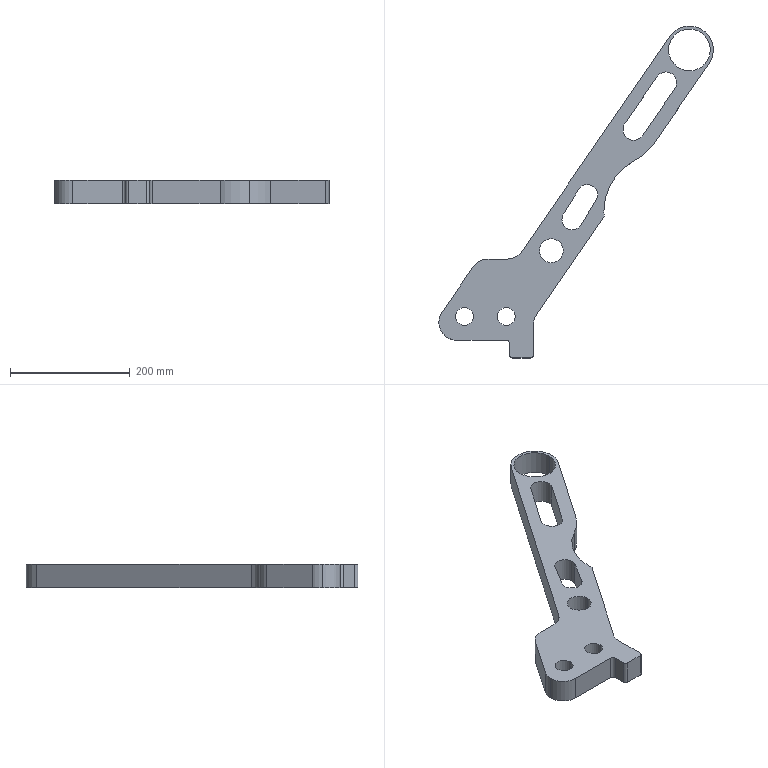Part | SolidWorks | features Extrusion 1 | 1 solid | 41 faces | box 459.333 x 555.5 x 40 mm | volume 1753830 mm3 | cylinder 26 | plane 15 | commonest cylinder face diameters 60 x5 30 x4 10 x3 35.817 x3 34.433 x2 40 x2
STEP:
#1=CARTESIAN_POINT('',(136223.495,-173373.447,40.));
#2=VERTEX_POINT('',#1);
#3=CARTESIAN_POINT('',(136220.343,-173383.593,40.));
#4=VERTEX_POINT('',#3);
#5=CARTESIAN_POINT('',(136238.252,-173383.593,40.));
#6=DIRECTION('',(0.,0.,1.));
#7=DIRECTION('',(1.,0.,0.));
#8=AXIS2_PLACEMENT_3D('',#5,#6,#7);
#9=CIRCLE('',#8,17.909);
#10=EDGE_CURVE('',#2,#4,#9,.T.);
#11=ORIENTED_EDGE('',*,*,#10,.T.);
#12=CARTESIAN_POINT('',(136220.343,-173383.593,0.));
#13=VERTEX_POINT('',#12);
#14=CARTESIAN_POINT('',(136220.343,-173383.593,40.));
#15=DIRECTION('',(0.,0.,-1.));
#16=VECTOR('',#15,1000.);
#17=LINE('',#14,#16);
#18=EDGE_CURVE('',#4,#13,#17,.T.);
#19=ORIENTED_EDGE('',*,*,#18,.T.);
#20=CARTESIAN_POINT('',(136223.495,-173373.447,0.));
#21=VERTEX_POINT('',#20);
#22=CARTESIAN_POINT('',(136238.252,-173383.593,0.));
#23=DIRECTION('',(0.,0.,1.));
#24=DIRECTION('',(1.,0.,0.));
#25=AXIS2_PLACEMENT_3D('',#22,#23,#24);
#26=CIRCLE('',#25,17.909);
#27=EDGE_CURVE('',#21,#13,#26,.T.);
#28=ORIENTED_EDGE('',*,*,#27,.F.);
#29=CARTESIAN_POINT('',(136223.495,-173373.447,40.));
#30=DIRECTION('',(0.,0.,-1.));
#31=VECTOR('',#30,1000.);
#32=LINE('',#29,#31);
#33=EDGE_CURVE('',#2,#21,#32,.T.);
#34=ORIENTED_EDGE('',*,*,#33,.F.);
#35=EDGE_LOOP('',(#11,#19,#28,#34));
#36=FACE_OUTER_BOUND('',#35,.T.);
#37=CARTESIAN_POINT('',(136238.252,-173383.593,40.));
#38=DIRECTION('',(0.,0.,-1.));
#39=DIRECTION('',(-1.,0.,0.));
#40=AXIS2_PLACEMENT_3D('',#37,#38,#39);
#41=CYLINDRICAL_SURFACE('',#40,17.909);
#42=ADVANCED_FACE('',(#36),#41,.F.);
#43=CARTESIAN_POINT('',(136121.227,-173524.21,40.));
#44=VERTEX_POINT('',#43);
#45=CARTESIAN_POINT('',(136118.026,-173534.208,40.));
#46=VERTEX_POINT('',#45);
#47=CARTESIAN_POINT('',(136135.243,-173534.208,40.));
#48=DIRECTION('',(0.,0.,1.));
#49=DIRECTION('',(1.,0.,0.));
#50=AXIS2_PLACEMENT_3D('',#47,#48,#49);
#51=CIRCLE('',#50,17.217);
#52=EDGE_CURVE('',#44,#46,#51,.T.);
#53=ORIENTED_EDGE('',*,*,#52,.T.);
#54=CARTESIAN_POINT('',(136118.026,-173534.208,0.));
#55=VERTEX_POINT('',#54);
#56=CARTESIAN_POINT('',(136118.026,-173534.208,40.));
#57=DIRECTION('',(0.,0.,-1.));
#58=VECTOR('',#57,1000.);
#59=LINE('',#56,#58);
#60=EDGE_CURVE('',#46,#55,#59,.T.);
#61=ORIENTED_EDGE('',*,*,#60,.T.);
#62=CARTESIAN_POINT('',(136121.227,-173524.21,0.));
#63=VERTEX_POINT('',#62);
#64=CARTESIAN_POINT('',(136135.243,-173534.208,0.));
#65=DIRECTION('',(0.,0.,1.));
#66=DIRECTION('',(1.,0.,0.));
#67=AXIS2_PLACEMENT_3D('',#64,#65,#66);
#68=CIRCLE('',#67,17.217);
#69=EDGE_CURVE('',#63,#55,#68,.T.);
#70=ORIENTED_EDGE('',*,*,#69,.F.);
#71=CARTESIAN_POINT('',(136121.227,-173524.21,40.));
#72=DIRECTION('',(0.,0.,-1.));
#73=VECTOR('',#72,1000.);
#74=LINE('',#71,#73);
#75=EDGE_CURVE('',#44,#63,#74,.T.);
#76=ORIENTED_EDGE('',*,*,#75,.F.);
#77=EDGE_LOOP('',(#53,#61,#70,#76));
#78=FACE_OUTER_BOUND('',#77,.T.);
#79=CARTESIAN_POINT('',(136135.243,-173534.208,40.));
#80=DIRECTION('',(0.,0.,-1.));
#81=DIRECTION('',(-1.,0.,0.));
#82=AXIS2_PLACEMENT_3D('',#79,#80,#81);
#83=CYLINDRICAL_SURFACE('',#82,17.217);
#84=ADVANCED_FACE('',(#78),#83,.F.);
#85=CARTESIAN_POINT('',(136296.441,-173250.292,40.));
#86=VERTEX_POINT('',#85);
#87=CARTESIAN_POINT('',(136366.441,-173250.292,40.));
#88=VERTEX_POINT('',#87);
#89=CARTESIAN_POINT('',(136331.441,-173250.292,40.));
#90=DIRECTION('',(0.,0.,1.));
#91=DIRECTION('',(1.,0.,0.));
#92=AXIS2_PLACEMENT_3D('',#89,#90,#91);
#93=CIRCLE('',#92,35.);
#94=EDGE_CURVE('',#86,#88,#93,.T.);
#95=ORIENTED_EDGE('',*,*,#94,.T.);
#96=CARTESIAN_POINT('',(136366.441,-173250.292,0.));
#97=VERTEX_POINT('',#96);
#98=CARTESIAN_POINT('',(136366.441,-173250.292,40.));
#99=DIRECTION('',(0.,0.,-1.));
#100=VECTOR('',#99,1000.);
#101=LINE('',#98,#100);
#102=EDGE_CURVE('',#88,#97,#101,.T.);
#103=ORIENTED_EDGE('',*,*,#102,.T.);
#104=CARTESIAN_POINT('',(136296.441,-173250.292,0.));
#105=VERTEX_POINT('',#104);
#106=CARTESIAN_POINT('',(136331.441,-173250.292,0.));
#107=DIRECTION('',(0.,0.,1.));
#108=DIRECTION('',(1.,0.,0.));
#109=AXIS2_PLACEMENT_3D('',#106,#107,#108);
#110=CIRCLE('',#109,35.);
#111=EDGE_CURVE('',#105,#97,#110,.T.);
#112=ORIENTED_EDGE('',*,*,#111,.F.);
#113=CARTESIAN_POINT('',(136296.441,-173250.292,40.));
#114=DIRECTION('',(0.,0.,-1.));
#115=VECTOR('',#114,1000.);
#116=LINE('',#113,#115);
#117=EDGE_CURVE('',#86,#105,#116,.T.);
#118=ORIENTED_EDGE('',*,*,#117,.F.);
#119=EDGE_LOOP('',(#95,#103,#112,#118));
#120=FACE_OUTER_BOUND('',#119,.T.);
#121=CARTESIAN_POINT('',(136331.441,-173250.292,40.));
#122=DIRECTION('',(0.,0.,-1.));
#123=DIRECTION('',(-1.,0.,0.));
#124=AXIS2_PLACEMENT_3D('',#121,#122,#123);
#125=CYLINDRICAL_SURFACE('',#124,35.);
#126=ADVANCED_FACE('',(#120),#125,.F.);
#127=CARTESIAN_POINT('',(136080.441,-173586.292,40.));
#128=VERTEX_POINT('',#127);
#129=CARTESIAN_POINT('',(136120.441,-173586.292,40.));
#130=VERTEX_POINT('',#129);
#131=CARTESIAN_POINT('',(136100.441,-173586.292,40.));
#132=DIRECTION('',(0.,0.,1.));
#133=DIRECTION('',(1.,0.,0.));
#134=AXIS2_PLACEMENT_3D('',#131,#132,#133);
#135=CIRCLE('',#134,20.);
#136=EDGE_CURVE('',#128,#130,#135,.T.);
#137=ORIENTED_EDGE('',*,*,#136,.T.);
#138=CARTESIAN_POINT('',(136120.441,-173586.292,0.));
#139=VERTEX_POINT('',#138);
#140=CARTESIAN_POINT('',(136120.441,-173586.292,40.));
#141=DIRECTION('',(0.,0.,-1.));
#142=VECTOR('',#141,1000.);
#143=LINE('',#140,#142);
#144=EDGE_CURVE('',#130,#139,#143,.T.);
#145=ORIENTED_EDGE('',*,*,#144,.T.);
#146=CARTESIAN_POINT('',(136080.441,-173586.292,0.));
#147=VERTEX_POINT('',#146);
#148=CARTESIAN_POINT('',(136100.441,-173586.292,0.));
#149=DIRECTION('',(0.,0.,1.));
#150=DIRECTION('',(1.,0.,0.));
#151=AXIS2_PLACEMENT_3D('',#148,#149,#150);
#152=CIRCLE('',#151,20.);
#153=EDGE_CURVE('',#147,#139,#152,.T.);
#154=ORIENTED_EDGE('',*,*,#153,.F.);
#155=CARTESIAN_POINT('',(136080.441,-173586.292,40.));
#156=DIRECTION('',(0.,0.,-1.));
#157=VECTOR('',#156,1000.);
#158=LINE('',#155,#157);
#159=EDGE_CURVE('',#128,#147,#158,.T.);
#160=ORIENTED_EDGE('',*,*,#159,.F.);
#161=EDGE_LOOP('',(#137,#145,#154,#160));
#162=FACE_OUTER_BOUND('',#161,.T.);
#163=CARTESIAN_POINT('',(136100.441,-173586.292,40.));
#164=DIRECTION('',(0.,0.,-1.));
#165=DIRECTION('',(-1.,0.,0.));
#166=AXIS2_PLACEMENT_3D('',#163,#164,#165);
#167=CYLINDRICAL_SURFACE('',#166,20.);
#168=ADVANCED_FACE('',(#162),#167,.F.);
#169=CARTESIAN_POINT('',(135939.816,-173696.292,40.));
#170=VERTEX_POINT('',#169);
#171=CARTESIAN_POINT('',(135969.816,-173696.292,40.));
#172=VERTEX_POINT('',#171);
#173=CARTESIAN_POINT('',(135954.816,-173696.292,40.));
#174=DIRECTION('',(0.,0.,1.));
#175=DIRECTION('',(1.,0.,0.));
#176=AXIS2_PLACEMENT_3D('',#173,#174,#175);
#177=CIRCLE('',#176,15.);
#178=EDGE_CURVE('',#170,#172,#177,.T.);
#179=ORIENTED_EDGE('',*,*,#178,.T.);
#180=CARTESIAN_POINT('',(135969.816,-173696.292,0.));
#181=VERTEX_POINT('',#180);
#182=CARTESIAN_POINT('',(135969.816,-173696.292,40.));
#183=DIRECTION('',(0.,0.,-1.));
#184=VECTOR('',#183,1000.);
#185=LINE('',#182,#184);
#186=EDGE_CURVE('',#172,#181,#185,.T.);
#187=ORIENTED_EDGE('',*,*,#186,.T.);
#188=CARTESIAN_POINT('',(135939.816,-173696.292,0.));
#189=VERTEX_POINT('',#188);
#190=CARTESIAN_POINT('',(135954.816,-173696.292,0.));
#191=DIRECTION('',(0.,0.,1.));
#192=DIRECTION('',(1.,0.,0.));
#193=AXIS2_PLACEMENT_3D('',#190,#191,#192);
#194=CIRCLE('',#193,15.);
#195=EDGE_CURVE('',#189,#181,#194,.T.);
#196=ORIENTED_EDGE('',*,*,#195,.F.);
#197=CARTESIAN_POINT('',(135939.816,-173696.292,40.));
#198=DIRECTION('',(0.,0.,-1.));
#199=VECTOR('',#198,1000.);
#200=LINE('',#197,#199);
#201=EDGE_CURVE('',#170,#189,#200,.T.);
#202=ORIENTED_EDGE('',*,*,#201,.F.);
#203=EDGE_LOOP('',(#179,#187,#196,#202));
#204=FACE_OUTER_BOUND('',#203,.T.);
#205=CARTESIAN_POINT('',(135954.816,-173696.292,40.));
#206=DIRECTION('',(0.,0.,-1.));
#207=DIRECTION('',(-1.,0.,0.));
#208=AXIS2_PLACEMENT_3D('',#205,#206,#207);
#209=CYLINDRICAL_SURFACE('',#208,15.);
#210=ADVANCED_FACE('',(#204),#209,.F.);
#211=CARTESIAN_POINT('',(136009.816,-173696.292,40.));
#212=VERTEX_POINT('',#211);
#213=CARTESIAN_POINT('',(136039.816,-173696.292,40.));
#214=VERTEX_POINT('',#213);
#215=CARTESIAN_POINT('',(136024.816,-173696.292,40.));
#216=DIRECTION('',(0.,0.,1.));
#217=DIRECTION('',(1.,0.,0.));
#218=AXIS2_PLACEMENT_3D('',#215,#216,#217);
#219=CIRCLE('',#218,15.);
#220=EDGE_CURVE('',#212,#214,#219,.T.);
#221=ORIENTED_EDGE('',*,*,#220,.T.);
#222=CARTESIAN_POINT('',(136039.816,-173696.292,0.));
#223=VERTEX_POINT('',#222);
#224=CARTESIAN_POINT('',(136039.816,-173696.292,40.));
#225=DIRECTION('',(0.,0.,-1.));
#226=VECTOR('',#225,1000.);
#227=LINE('',#224,#226);
#228=EDGE_CURVE('',#214,#223,#227,.T.);
#229=ORIENTED_EDGE('',*,*,#228,.T.);
#230=CARTESIAN_POINT('',(136009.816,-173696.292,0.));
#231=VERTEX_POINT('',#230);
#232=CARTESIAN_POINT('',(136024.816,-173696.292,0.));
#233=DIRECTION('',(0.,0.,1.));
#234=DIRECTION('',(1.,0.,0.));
#235=AXIS2_PLACEMENT_3D('',#232,#233,#234);
#236=CIRCLE('',#235,15.);
#237=EDGE_CURVE('',#231,#223,#236,.T.);
#238=ORIENTED_EDGE('',*,*,#237,.F.);
#239=CARTESIAN_POINT('',(136009.816,-173696.292,40.));
#240=DIRECTION('',(0.,0.,-1.));
#241=VECTOR('',#240,1000.);
#242=LINE('',#239,#241);
#243=EDGE_CURVE('',#212,#231,#242,.T.);
#244=ORIENTED_EDGE('',*,*,#243,.F.);
#245=EDGE_LOOP('',(#221,#229,#238,#244));
#246=FACE_OUTER_BOUND('',#245,.T.);
#247=CARTESIAN_POINT('',(136024.816,-173696.292,40.));
#248=DIRECTION('',(0.,0.,-1.));
#249=DIRECTION('',(-1.,0.,0.));
#250=AXIS2_PLACEMENT_3D('',#247,#248,#249);
#251=CYLINDRICAL_SURFACE('',#250,15.);
#252=ADVANCED_FACE('',(#246),#251,.F.);
#253=CARTESIAN_POINT('',(136188.379,-173519.712,40.));
#254=VERTEX_POINT('',#253);
#255=CARTESIAN_POINT('',(136238.252,-173436.604,40.));
#256=VERTEX_POINT('',#255);
#257=CARTESIAN_POINT('',(136282.56,-173519.712,40.));
#258=DIRECTION('',(0.,0.,-1.));
#259=DIRECTION('',(-1.,0.,0.));
#260=AXIS2_PLACEMENT_3D('',#257,#258,#259);
#261=CIRCLE('',#260,94.181);
#262=EDGE_CURVE('',#254,#256,#261,.T.);
#263=ORIENTED_EDGE('',*,*,#262,.F.);
#264=CARTESIAN_POINT('',(136188.379,-173519.712,0.));
#265=VERTEX_POINT('',#264);
#266=CARTESIAN_POINT('',(136188.379,-173519.712,40.));
#267=DIRECTION('',(0.,0.,-1.));
#268=VECTOR('',#267,1000.);
#269=LINE('',#266,#268);
#270=EDGE_CURVE('',#254,#265,#269,.T.);
#271=ORIENTED_EDGE('',*,*,#270,.T.);
#272=CARTESIAN_POINT('',(136238.252,-173436.604,0.));
#273=VERTEX_POINT('',#272);
#274=CARTESIAN_POINT('',(136282.56,-173519.712,0.));
#275=DIRECTION('',(0.,0.,-1.));
#276=DIRECTION('',(-1.,0.,0.));
#277=AXIS2_PLACEMENT_3D('',#274,#275,#276);
#278=CIRCLE('',#277,94.181);
#279=EDGE_CURVE('',#265,#273,#278,.T.);
#280=ORIENTED_EDGE('',*,*,#279,.T.);
#281=CARTESIAN_POINT('',(136238.252,-173436.604,40.));
#282=DIRECTION('',(0.,0.,-1.));
#283=VECTOR('',#282,1000.);
#284=LINE('',#281,#283);
#285=EDGE_CURVE('',#256,#273,#284,.T.);
#286=ORIENTED_EDGE('',*,*,#285,.F.);
#287=EDGE_LOOP('',(#263,#271,#280,#286));
#288=FACE_OUTER_BOUND('',#287,.T.);
#289=CARTESIAN_POINT('',(136282.56,-173519.712,40.));
#290=DIRECTION('',(0.,0.,-1.));
#291=DIRECTION('',(-1.,0.,0.));
#292=AXIS2_PLACEMENT_3D('',#289,#290,#291);
#293=CYLINDRICAL_SURFACE('',#292,94.181);
#294=ADVANCED_FACE('',(#288),#293,.F.);
#295=CARTESIAN_POINT('',(135912.108,-173706.292,40.));
#296=VERTEX_POINT('',#295);
#297=CARTESIAN_POINT('',(135942.108,-173736.292,40.));
#298=VERTEX_POINT('',#297);
#299=CARTESIAN_POINT('',(135942.108,-173706.292,40.));
#300=DIRECTION('',(0.,0.,1.));
#301=DIRECTION('',(1.,0.,0.));
#302=AXIS2_PLACEMENT_3D('',#299,#300,#301);
#303=CIRCLE('',#302,30.);
#304=EDGE_CURVE('',#296,#298,#303,.T.);
#305=ORIENTED_EDGE('',*,*,#304,.F.);
#306=CARTESIAN_POINT('',(135912.108,-173706.292,0.));
#307=VERTEX_POINT('',#306);
#308=CARTESIAN_POINT('',(135912.108,-173706.292,40.));
#309=DIRECTION('',(0.,0.,-1.));
#310=VECTOR('',#309,1000.);
#311=LINE('',#308,#310);
#312=EDGE_CURVE('',#296,#307,#311,.T.);
#313=ORIENTED_EDGE('',*,*,#312,.T.);
#314=CARTESIAN_POINT('',(135942.108,-173736.292,0.));
#315=VERTEX_POINT('',#314);
#316=CARTESIAN_POINT('',(135942.108,-173706.292,0.));
#317=DIRECTION('',(0.,0.,1.));
#318=DIRECTION('',(1.,0.,0.));
#319=AXIS2_PLACEMENT_3D('',#316,#317,#318);
#320=CIRCLE('',#319,30.);
#321=EDGE_CURVE('',#307,#315,#320,.T.);
#322=ORIENTED_EDGE('',*,*,#321,.T.);
#323=CARTESIAN_POINT('',(135942.108,-173736.292,40.));
#324=DIRECTION('',(0.,0.,-1.));
#325=VECTOR('',#324,1000.);
#326=LINE('',#323,#325);
#327=EDGE_CURVE('',#298,#315,#326,.T.);
#328=ORIENTED_EDGE('',*,*,#327,.F.);
#329=EDGE_LOOP('',(#305,#313,#322,#328));
#330=FACE_OUTER_BOUND('',#329,.T.);
#331=CARTESIAN_POINT('',(135942.108,-173706.292,40.));
#332=DIRECTION('',(0.,0.,-1.));
#333=DIRECTION('',(-1.,0.,0.));
#334=AXIS2_PLACEMENT_3D('',#331,#332,#333);
#335=CYLINDRICAL_SURFACE('',#334,30.);
#336=ADVANCED_FACE('',(#330),#335,.T.);
#337=ORIENTED_EDGE('',*,*,#136,.F.);
#338=CARTESIAN_POINT('',(136100.441,-173586.292,40.));
#339=DIRECTION('',(0.,0.,1.));
#340=DIRECTION('',(1.,0.,0.));
#341=AXIS2_PLACEMENT_3D('',#338,#339,#340);
#342=CIRCLE('',#341,20.);
#343=EDGE_CURVE('',#130,#128,#342,.T.);
#344=ORIENTED_EDGE('',*,*,#343,.F.);
#345=EDGE_LOOP('',(#337,#344));
#346=FACE_BOUND('',#345,.T.);
#347=ORIENTED_EDGE('',*,*,#220,.F.);
#348=CARTESIAN_POINT('',(136024.816,-173696.292,40.));
#349=DIRECTION('',(0.,0.,1.));
#350=DIRECTION('',(1.,0.,0.));
#351=AXIS2_PLACEMENT_3D('',#348,#349,#350);
#352=CIRCLE('',#351,15.);
#353=EDGE_CURVE('',#214,#212,#352,.T.);
#354=ORIENTED_EDGE('',*,*,#353,.F.);
#355=EDGE_LOOP('',(#347,#354));
#356=FACE_BOUND('',#355,.T.);
#357=CARTESIAN_POINT('',(136364.403,-173272.954,40.));
#358=VERTEX_POINT('',#357);
#359=CARTESIAN_POINT('',(136298.479,-173227.631,40.));
#360=VERTEX_POINT('',#359);
#361=CARTESIAN_POINT('',(136331.441,-173250.292,40.));
#362=DIRECTION('',(0.,0.,1.));
#363=DIRECTION('',(1.,0.,0.));
#364=AXIS2_PLACEMENT_3D('',#361,#362,#363);
#365=CIRCLE('',#364,40.);
#366=EDGE_CURVE('',#358,#360,#365,.T.);
#367=ORIENTED_EDGE('',*,*,#366,.T.);
#368=CARTESIAN_POINT('',(136051.215,-173587.288,40.));
#369=VERTEX_POINT('',#368);
#370=CARTESIAN_POINT('',(136298.479,-173227.631,40.));
#371=DIRECTION('',(-0.5665,-0.824,0.));
#372=VECTOR('',#371,1000.);
#373=LINE('',#370,#372);
#374=EDGE_CURVE('',#360,#369,#373,.T.);
#375=ORIENTED_EDGE('',*,*,#374,.T.);
#376=CARTESIAN_POINT('',(136026.494,-173600.292,40.));
#377=VERTEX_POINT('',#376);
#378=CARTESIAN_POINT('',(136026.494,-173570.292,40.));
#379=DIRECTION('',(0.,0.,-1.));
#380=DIRECTION('',(1.,0.,0.));
#381=AXIS2_PLACEMENT_3D('',#378,#379,#380);
#382=CIRCLE('',#381,30.);
#383=EDGE_CURVE('',#369,#377,#382,.T.);
#384=ORIENTED_EDGE('',*,*,#383,.T.);
#385=CARTESIAN_POINT('',(135994.358,-173600.292,40.));
#386=VERTEX_POINT('',#385);
#387=CARTESIAN_POINT('',(135994.358,-173600.292,40.));
#388=DIRECTION('',(-1.,0.,0.));
#389=VECTOR('',#388,1000.);
#390=LINE('',#387,#389);
#391=EDGE_CURVE('',#377,#386,#390,.T.);
#392=ORIENTED_EDGE('',*,*,#391,.T.);
#393=CARTESIAN_POINT('',(135969.637,-173613.297,40.));
#394=VERTEX_POINT('',#393);
#395=CARTESIAN_POINT('',(135994.358,-173630.292,40.));
#396=DIRECTION('',(0.,0.,1.));
#397=DIRECTION('',(1.,0.,0.));
#398=AXIS2_PLACEMENT_3D('',#395,#396,#397);
#399=CIRCLE('',#398,30.);
#400=EDGE_CURVE('',#386,#394,#399,.T.);
#401=ORIENTED_EDGE('',*,*,#400,.T.);
#402=CARTESIAN_POINT('',(135917.387,-173689.297,40.));
#403=VERTEX_POINT('',#402);
#404=CARTESIAN_POINT('',(135969.637,-173613.297,40.));
#405=DIRECTION('',(-0.5665,-0.824,0.));
#406=VECTOR('',#405,1000.);
#407=LINE('',#404,#406);
#408=EDGE_CURVE('',#394,#403,#407,.T.);
#409=ORIENTED_EDGE('',*,*,#408,.T.);
#410=CARTESIAN_POINT('',(135942.108,-173706.292,40.));
#411=DIRECTION('',(0.,0.,1.));
#412=DIRECTION('',(1.,0.,0.));
#413=AXIS2_PLACEMENT_3D('',#410,#411,#412);
#414=CIRCLE('',#413,30.);
#415=EDGE_CURVE('',#403,#296,#414,.T.);
#416=ORIENTED_EDGE('',*,*,#415,.T.);
#417=ORIENTED_EDGE('',*,*,#304,.T.);
#418=CARTESIAN_POINT('',(136025.441,-173736.292,40.));
#419=VERTEX_POINT('',#418);
#420=CARTESIAN_POINT('',(135942.108,-173736.292,40.));
#421=DIRECTION('',(1.,0.,0.));
#422=VECTOR('',#421,1000.);
#423=LINE('',#420,#422);
#424=EDGE_CURVE('',#298,#419,#423,.T.);
#425=ORIENTED_EDGE('',*,*,#424,.T.);
#426=CARTESIAN_POINT('',(136030.441,-173741.292,40.));
#427=VERTEX_POINT('',#426);
#428=CARTESIAN_POINT('',(136025.441,-173741.292,40.));
#429=DIRECTION('',(0.,0.,-1.));
#430=DIRECTION('',(1.,0.,0.));
#431=AXIS2_PLACEMENT_3D('',#428,#429,#430);
#432=CIRCLE('',#431,5.);
#433=EDGE_CURVE('',#419,#427,#432,.T.);
#434=ORIENTED_EDGE('',*,*,#433,.T.);
#435=CARTESIAN_POINT('',(136030.441,-173760.792,40.));
#436=VERTEX_POINT('',#435);
#437=CARTESIAN_POINT('',(136030.441,-173760.792,40.));
#438=DIRECTION('',(0.,-1.,0.));
#439=VECTOR('',#438,1000.);
#440=LINE('',#437,#439);
#441=EDGE_CURVE('',#427,#436,#440,.T.);
#442=ORIENTED_EDGE('',*,*,#441,.T.);
#443=CARTESIAN_POINT('',(136035.441,-173765.792,40.));
#444=VERTEX_POINT('',#443);
#445=CARTESIAN_POINT('',(136035.441,-173760.792,40.));
#446=DIRECTION('',(0.,0.,1.));
#447=DIRECTION('',(1.,0.,0.));
#448=AXIS2_PLACEMENT_3D('',#445,#446,#447);
#449=CIRCLE('',#448,5.);
#450=EDGE_CURVE('',#436,#444,#449,.T.);
#451=ORIENTED_EDGE('',*,*,#450,.T.);
#452=CARTESIAN_POINT('',(136065.441,-173765.792,40.));
#453=VERTEX_POINT('',#452);
#454=CARTESIAN_POINT('',(136035.441,-173765.792,40.));
#455=DIRECTION('',(1.,0.,0.));
#456=VECTOR('',#455,1000.);
#457=LINE('',#454,#456);
#458=EDGE_CURVE('',#444,#453,#457,.T.);
#459=ORIENTED_EDGE('',*,*,#458,.T.);
#460=CARTESIAN_POINT('',(136070.441,-173760.792,40.));
#461=VERTEX_POINT('',#460);
#462=CARTESIAN_POINT('',(136065.441,-173760.792,40.));
#463=DIRECTION('',(0.,0.,1.));
#464=DIRECTION('',(1.,0.,0.));
#465=AXIS2_PLACEMENT_3D('',#462,#463,#464);
#466=CIRCLE('',#465,5.);
#467=EDGE_CURVE('',#453,#461,#466,.T.);
#468=ORIENTED_EDGE('',*,*,#467,.T.);
#469=CARTESIAN_POINT('',(136070.441,-173709.852,40.));
#470=VERTEX_POINT('',#469);
#471=CARTESIAN_POINT('',(136070.441,-173760.792,40.));
#472=DIRECTION('',(0.,1.,0.));
#473=VECTOR('',#472,1000.);
#474=LINE('',#471,#473);
#475=EDGE_CURVE('',#461,#470,#474,.T.);
#476=ORIENTED_EDGE('',*,*,#475,.T.);
#477=CARTESIAN_POINT('',(136075.72,-173692.856,40.));
#478=VERTEX_POINT('',#477);
#479=CARTESIAN_POINT('',(136100.441,-173709.852,40.));
#480=DIRECTION('',(0.,0.,-1.));
#481=DIRECTION('',(1.,0.,0.));
#482=AXIS2_PLACEMENT_3D('',#479,#480,#481);
#483=CIRCLE('',#482,30.);
#484=EDGE_CURVE('',#470,#478,#483,.T.);
#485=ORIENTED_EDGE('',*,*,#484,.T.);
#486=CARTESIAN_POINT('',(136188.781,-173528.403,40.));
#487=VERTEX_POINT('',#486);
#488=CARTESIAN_POINT('',(136188.781,-173528.403,40.));
#489=DIRECTION('',(0.5665,0.824,0.));
#490=VECTOR('',#489,1000.);
#491=LINE('',#488,#490);
#492=EDGE_CURVE('',#478,#487,#491,.T.);
#493=ORIENTED_EDGE('',*,*,#492,.T.);
#494=CARTESIAN_POINT('',(136282.56,-173519.712,40.));
#495=DIRECTION('',(0.,0.,-1.));
#496=DIRECTION('',(-1.,0.,0.));
#497=AXIS2_PLACEMENT_3D('',#494,#495,#496);
#498=CIRCLE('',#497,94.181);
#499=EDGE_CURVE('',#487,#254,#498,.T.);
#500=ORIENTED_EDGE('',*,*,#499,.T.);
#501=ORIENTED_EDGE('',*,*,#262,.T.);
#502=CARTESIAN_POINT('',(136273.61,-173405.015,40.));
#503=VERTEX_POINT('',#502);
#504=CARTESIAN_POINT('',(136191.206,-173348.362,40.));
#505=DIRECTION('',(0.,0.,1.));
#506=DIRECTION('',(1.,0.,0.));
#507=AXIS2_PLACEMENT_3D('',#504,#505,#506);
#508=CIRCLE('',#507,100.);
#509=EDGE_CURVE('',#256,#503,#508,.T.);
#510=ORIENTED_EDGE('',*,*,#509,.T.);
#511=CARTESIAN_POINT('',(136364.403,-173272.954,40.));
#512=DIRECTION('',(0.5665,0.824,0.));
#513=VECTOR('',#512,1000.);
#514=LINE('',#511,#513);
#515=EDGE_CURVE('',#503,#358,#514,.T.);
#516=ORIENTED_EDGE('',*,*,#515,.T.);
#517=EDGE_LOOP('',(#367,#375,#384,#392,#401,#409,#416,#417,#425,#434,#442,#451,#459,#468,#476,#485,#493,#500,#501,#510,#516));
#518=FACE_OUTER_BOUND('',#517,.T.);
#519=ORIENTED_EDGE('',*,*,#178,.F.);
#520=CARTESIAN_POINT('',(135954.816,-173696.292,40.));
#521=DIRECTION('',(0.,0.,1.));
#522=DIRECTION('',(1.,0.,0.));
#523=AXIS2_PLACEMENT_3D('',#520,#521,#522);
#524=CIRCLE('',#523,15.);
#525=EDGE_CURVE('',#172,#170,#524,.T.);
#526=ORIENTED_EDGE('',*,*,#525,.F.);
#527=EDGE_LOOP('',(#519,#526));
#528=FACE_BOUND('',#527,.T.);
#529=ORIENTED_EDGE('',*,*,#94,.F.);
#530=CARTESIAN_POINT('',(136331.441,-173250.292,40.));
#531=DIRECTION('',(0.,0.,1.));
#532=DIRECTION('',(1.,0.,0.));
#533=AXIS2_PLACEMENT_3D('',#530,#531,#532);
#534=CIRCLE('',#533,35.);
#535=EDGE_CURVE('',#88,#86,#534,.T.);
#536=ORIENTED_EDGE('',*,*,#535,.F.);
#537=EDGE_LOOP('',(#529,#536));
#538=FACE_BOUND('',#537,.T.);
#539=CARTESIAN_POINT('',(136150.474,-173542.235,40.));
#540=VERTEX_POINT('',#539);
#541=CARTESIAN_POINT('',(136175.848,-173500.774,40.));
#542=VERTEX_POINT('',#541);
#543=CARTESIAN_POINT('',(136150.474,-173542.235,40.));
#544=DIRECTION('',(0.522,0.8529,0.));
#545=VECTOR('',#544,1000.);
#546=LINE('',#543,#545);
#547=EDGE_CURVE('',#540,#542,#546,.T.);
#548=ORIENTED_EDGE('',*,*,#547,.F.);
#549=CARTESIAN_POINT('',(136135.243,-173534.208,40.));
#550=DIRECTION('',(0.,0.,1.));
#551=DIRECTION('',(1.,0.,0.));
#552=AXIS2_PLACEMENT_3D('',#549,#550,#551);
#553=CIRCLE('',#552,17.217);
#554=EDGE_CURVE('',#46,#540,#553,.T.);
#555=ORIENTED_EDGE('',*,*,#554,.F.);
#556=ORIENTED_EDGE('',*,*,#52,.F.);
#557=CARTESIAN_POINT('',(136146.694,-173482.736,40.));
#558=VERTEX_POINT('',#557);
#559=CARTESIAN_POINT('',(136121.227,-173524.21,40.));
#560=DIRECTION('',(-0.5233,-0.8522,0.));
#561=VECTOR('',#560,1000.);
#562=LINE('',#559,#561);
#563=EDGE_CURVE('',#558,#44,#562,.T.);
#564=ORIENTED_EDGE('',*,*,#563,.F.);
#565=CARTESIAN_POINT('',(136160.639,-173492.777,40.));
#566=DIRECTION('',(0.,0.,1.));
#567=DIRECTION('',(1.,0.,0.));
#568=AXIS2_PLACEMENT_3D('',#565,#566,#567);
#569=CIRCLE('',#568,17.184);
#570=EDGE_CURVE('',#542,#558,#569,.T.);
#571=ORIENTED_EDGE('',*,*,#570,.F.);
#572=EDGE_LOOP('',(#548,#555,#556,#564,#571));
#573=FACE_BOUND('',#572,.T.);
#574=CARTESIAN_POINT('',(136253.009,-173393.739,40.));
#575=VERTEX_POINT('',#574);
#576=CARTESIAN_POINT('',(136306.988,-173315.224,40.));
#577=VERTEX_POINT('',#576);
#578=CARTESIAN_POINT('',(136253.009,-173393.739,40.));
#579=DIRECTION('',(0.5665,0.824,0.));
#580=VECTOR('',#579,1000.);
#581=LINE('',#578,#580);
#582=EDGE_CURVE('',#575,#577,#581,.T.);
#583=ORIENTED_EDGE('',*,*,#582,.F.);
#584=CARTESIAN_POINT('',(136238.252,-173383.593,40.));
#585=DIRECTION('',(0.,0.,1.));
#586=DIRECTION('',(1.,0.,0.));
#587=AXIS2_PLACEMENT_3D('',#584,#585,#586);
#588=CIRCLE('',#587,17.909);
#589=EDGE_CURVE('',#4,#575,#588,.T.);
#590=ORIENTED_EDGE('',*,*,#589,.F.);
#591=ORIENTED_EDGE('',*,*,#10,.F.);
#592=CARTESIAN_POINT('',(136277.474,-173294.933,40.));
#593=VERTEX_POINT('',#592);
#594=CARTESIAN_POINT('',(136223.495,-173373.447,40.));
#595=DIRECTION('',(-0.5665,-0.824,0.));
#596=VECTOR('',#595,1000.);
#597=LINE('',#594,#596);
#598=EDGE_CURVE('',#593,#2,#597,.T.);
#599=ORIENTED_EDGE('',*,*,#598,.F.);
#600=CARTESIAN_POINT('',(136292.231,-173305.078,40.));
#601=DIRECTION('',(0.,0.,1.));
#602=DIRECTION('',(1.,0.,0.));
#603=AXIS2_PLACEMENT_3D('',#600,#601,#602);
#604=CIRCLE('',#603,17.909);
#605=EDGE_CURVE('',#577,#593,#604,.T.);
#606=ORIENTED_EDGE('',*,*,#605,.F.);
#607=EDGE_LOOP('',(#583,#590,#591,#599,#606));
#608=FACE_BOUND('',#607,.T.);
#609=CARTESIAN_POINT('',(136331.441,-173250.292,40.));
#610=DIRECTION('',(0.,0.,1.));
#611=DIRECTION('',(1.,0.,0.));
#612=AXIS2_PLACEMENT_3D('',#609,#610,#611);
#613=PLANE('',#612);
#614=ADVANCED_FACE('',(#346,#356,#518,#528,#538,#573,#608),#613,.T.);
#615=ORIENTED_EDGE('',*,*,#69,.T.);
#616=CARTESIAN_POINT('',(136150.474,-173542.235,0.));
#617=VERTEX_POINT('',#616);
#618=CARTESIAN_POINT('',(136135.243,-173534.208,0.));
#619=DIRECTION('',(0.,0.,1.));
#620=DIRECTION('',(1.,0.,0.));
#621=AXIS2_PLACEMENT_3D('',#618,#619,#620);
#622=CIRCLE('',#621,17.217);
#623=EDGE_CURVE('',#55,#617,#622,.T.);
#624=ORIENTED_EDGE('',*,*,#623,.T.);
#625=CARTESIAN_POINT('',(136175.848,-173500.774,0.));
#626=VERTEX_POINT('',#625);
#627=CARTESIAN_POINT('',(136150.474,-173542.235,0.));
#628=DIRECTION('',(0.522,0.8529,0.));
#629=VECTOR('',#628,1000.);
#630=LINE('',#627,#629);
#631=EDGE_CURVE('',#617,#626,#630,.T.);
#632=ORIENTED_EDGE('',*,*,#631,.T.);
#633=CARTESIAN_POINT('',(136146.694,-173482.736,0.));
#634=VERTEX_POINT('',#633);
#635=CARTESIAN_POINT('',(136160.639,-173492.777,0.));
#636=DIRECTION('',(0.,0.,1.));
#637=DIRECTION('',(1.,0.,0.));
#638=AXIS2_PLACEMENT_3D('',#635,#636,#637);
#639=CIRCLE('',#638,17.184);
#640=EDGE_CURVE('',#626,#634,#639,.T.);
#641=ORIENTED_EDGE('',*,*,#640,.T.);
#642=CARTESIAN_POINT('',(136121.227,-173524.21,0.));
#643=DIRECTION('',(-0.5233,-0.8522,0.));
#644=VECTOR('',#643,1000.);
#645=LINE('',#642,#644);
#646=EDGE_CURVE('',#634,#63,#645,.T.);
#647=ORIENTED_EDGE('',*,*,#646,.T.);
#648=EDGE_LOOP('',(#615,#624,#632,#641,#647));
#649=FACE_BOUND('',#648,.T.);
#650=CARTESIAN_POINT('',(136364.403,-173272.954,0.));
#651=VERTEX_POINT('',#650);
#652=CARTESIAN_POINT('',(136298.479,-173227.631,0.));
#653=VERTEX_POINT('',#652);
#654=CARTESIAN_POINT('',(136331.441,-173250.292,0.));
#655=DIRECTION('',(0.,0.,1.));
#656=DIRECTION('',(1.,0.,0.));
#657=AXIS2_PLACEMENT_3D('',#654,#655,#656);
#658=CIRCLE('',#657,40.);
#659=EDGE_CURVE('',#651,#653,#658,.T.);
#660=ORIENTED_EDGE('',*,*,#659,.F.);
#661=CARTESIAN_POINT('',(136273.61,-173405.015,0.));
#662=VERTEX_POINT('',#661);
#663=CARTESIAN_POINT('',(136364.403,-173272.954,0.));
#664=DIRECTION('',(0.5665,0.824,0.));
#665=VECTOR('',#664,1000.);
#666=LINE('',#663,#665);
#667=EDGE_CURVE('',#662,#651,#666,.T.);
#668=ORIENTED_EDGE('',*,*,#667,.F.);
#669=CARTESIAN_POINT('',(136191.206,-173348.362,0.));
#670=DIRECTION('',(0.,0.,1.));
#671=DIRECTION('',(1.,0.,0.));
#672=AXIS2_PLACEMENT_3D('',#669,#670,#671);
#673=CIRCLE('',#672,100.);
#674=EDGE_CURVE('',#273,#662,#673,.T.);
#675=ORIENTED_EDGE('',*,*,#674,.F.);
#676=ORIENTED_EDGE('',*,*,#279,.F.);
#677=CARTESIAN_POINT('',(136188.781,-173528.403,0.));
#678=VERTEX_POINT('',#677);
#679=CARTESIAN_POINT('',(136282.56,-173519.712,0.));
#680=DIRECTION('',(0.,0.,-1.));
#681=DIRECTION('',(-1.,0.,0.));
#682=AXIS2_PLACEMENT_3D('',#679,#680,#681);
#683=CIRCLE('',#682,94.181);
#684=EDGE_CURVE('',#678,#265,#683,.T.);
#685=ORIENTED_EDGE('',*,*,#684,.F.);
#686=CARTESIAN_POINT('',(136075.72,-173692.856,0.));
#687=VERTEX_POINT('',#686);
#688=CARTESIAN_POINT('',(136188.781,-173528.403,0.));
#689=DIRECTION('',(0.5665,0.824,0.));
#690=VECTOR('',#689,1000.);
#691=LINE('',#688,#690);
#692=EDGE_CURVE('',#687,#678,#691,.T.);
#693=ORIENTED_EDGE('',*,*,#692,.F.);
#694=CARTESIAN_POINT('',(136070.441,-173709.852,0.));
#695=VERTEX_POINT('',#694);
#696=CARTESIAN_POINT('',(136100.441,-173709.852,0.));
#697=DIRECTION('',(0.,0.,-1.));
#698=DIRECTION('',(1.,0.,0.));
#699=AXIS2_PLACEMENT_3D('',#696,#697,#698);
#700=CIRCLE('',#699,30.);
#701=EDGE_CURVE('',#695,#687,#700,.T.);
#702=ORIENTED_EDGE('',*,*,#701,.F.);
#703=CARTESIAN_POINT('',(136070.441,-173760.792,0.));
#704=VERTEX_POINT('',#703);
#705=CARTESIAN_POINT('',(136070.441,-173760.792,0.));
#706=DIRECTION('',(0.,1.,0.));
#707=VECTOR('',#706,1000.);
#708=LINE('',#705,#707);
#709=EDGE_CURVE('',#704,#695,#708,.T.);
#710=ORIENTED_EDGE('',*,*,#709,.F.);
#711=CARTESIAN_POINT('',(136065.441,-173765.792,0.));
#712=VERTEX_POINT('',#711);
#713=CARTESIAN_POINT('',(136065.441,-173760.792,0.));
#714=DIRECTION('',(0.,0.,1.));
#715=DIRECTION('',(1.,0.,0.));
#716=AXIS2_PLACEMENT_3D('',#713,#714,#715);
#717=CIRCLE('',#716,5.);
#718=EDGE_CURVE('',#712,#704,#717,.T.);
#719=ORIENTED_EDGE('',*,*,#718,.F.);
#720=CARTESIAN_POINT('',(136035.441,-173765.792,0.));
#721=VERTEX_POINT('',#720);
#722=CARTESIAN_POINT('',(136035.441,-173765.792,0.));
#723=DIRECTION('',(1.,0.,0.));
#724=VECTOR('',#723,1000.);
#725=LINE('',#722,#724);
#726=EDGE_CURVE('',#721,#712,#725,.T.);
#727=ORIENTED_EDGE('',*,*,#726,.F.);
#728=CARTESIAN_POINT('',(136030.441,-173760.792,0.));
#729=VERTEX_POINT('',#728);
#730=CARTESIAN_POINT('',(136035.441,-173760.792,0.));
#731=DIRECTION('',(0.,0.,1.));
#732=DIRECTION('',(1.,0.,0.));
#733=AXIS2_PLACEMENT_3D('',#730,#731,#732);
#734=CIRCLE('',#733,5.);
#735=EDGE_CURVE('',#729,#721,#734,.T.);
#736=ORIENTED_EDGE('',*,*,#735,.F.);
#737=CARTESIAN_POINT('',(136030.441,-173741.292,0.));
#738=VERTEX_POINT('',#737);
#739=CARTESIAN_POINT('',(136030.441,-173760.792,0.));
#740=DIRECTION('',(0.,-1.,0.));
#741=VECTOR('',#740,1000.);
#742=LINE('',#739,#741);
#743=EDGE_CURVE('',#738,#729,#742,.T.);
#744=ORIENTED_EDGE('',*,*,#743,.F.);
#745=CARTESIAN_POINT('',(136025.441,-173736.292,0.));
#746=VERTEX_POINT('',#745);
#747=CARTESIAN_POINT('',(136025.441,-173741.292,0.));
#748=DIRECTION('',(0.,0.,-1.));
#749=DIRECTION('',(1.,0.,0.));
#750=AXIS2_PLACEMENT_3D('',#747,#748,#749);
#751=CIRCLE('',#750,5.);
#752=EDGE_CURVE('',#746,#738,#751,.T.);
#753=ORIENTED_EDGE('',*,*,#752,.F.);
#754=CARTESIAN_POINT('',(135942.108,-173736.292,0.));
#755=DIRECTION('',(1.,0.,0.));
#756=VECTOR('',#755,1000.);
#757=LINE('',#754,#756);
#758=EDGE_CURVE('',#315,#746,#757,.T.);
#759=ORIENTED_EDGE('',*,*,#758,.F.);
#760=ORIENTED_EDGE('',*,*,#321,.F.);
#761=CARTESIAN_POINT('',(135917.387,-173689.297,0.));
#762=VERTEX_POINT('',#761);
#763=CARTESIAN_POINT('',(135942.108,-173706.292,0.));
#764=DIRECTION('',(0.,0.,1.));
#765=DIRECTION('',(1.,0.,0.));
#766=AXIS2_PLACEMENT_3D('',#763,#764,#765);
#767=CIRCLE('',#766,30.);
#768=EDGE_CURVE('',#762,#307,#767,.T.);
#769=ORIENTED_EDGE('',*,*,#768,.F.);
#770=CARTESIAN_POINT('',(135969.637,-173613.297,0.));
#771=VERTEX_POINT('',#770);
#772=CARTESIAN_POINT('',(135969.637,-173613.297,0.));
#773=DIRECTION('',(-0.5665,-0.824,0.));
#774=VECTOR('',#773,1000.);
#775=LINE('',#772,#774);
#776=EDGE_CURVE('',#771,#762,#775,.T.);
#777=ORIENTED_EDGE('',*,*,#776,.F.);
#778=CARTESIAN_POINT('',(135994.358,-173600.292,0.));
#779=VERTEX_POINT('',#778);
#780=CARTESIAN_POINT('',(135994.358,-173630.292,0.));
#781=DIRECTION('',(0.,0.,1.));
#782=DIRECTION('',(1.,0.,0.));
#783=AXIS2_PLACEMENT_3D('',#780,#781,#782);
#784=CIRCLE('',#783,30.);
#785=EDGE_CURVE('',#779,#771,#784,.T.);
#786=ORIENTED_EDGE('',*,*,#785,.F.);
#787=CARTESIAN_POINT('',(136026.494,-173600.292,0.));
#788=VERTEX_POINT('',#787);
#789=CARTESIAN_POINT('',(135994.358,-173600.292,0.));
#790=DIRECTION('',(-1.,0.,0.));
#791=VECTOR('',#790,1000.);
#792=LINE('',#789,#791);
#793=EDGE_CURVE('',#788,#779,#792,.T.);
#794=ORIENTED_EDGE('',*,*,#793,.F.);
#795=CARTESIAN_POINT('',(136051.215,-173587.288,0.));
#796=VERTEX_POINT('',#795);
#797=CARTESIAN_POINT('',(136026.494,-173570.292,0.));
#798=DIRECTION('',(0.,0.,-1.));
#799=DIRECTION('',(1.,0.,0.));
#800=AXIS2_PLACEMENT_3D('',#797,#798,#799);
#801=CIRCLE('',#800,30.);
#802=EDGE_CURVE('',#796,#788,#801,.T.);
#803=ORIENTED_EDGE('',*,*,#802,.F.);
#804=CARTESIAN_POINT('',(136298.479,-173227.631,0.));
#805=DIRECTION('',(-0.5665,-0.824,0.));
#806=VECTOR('',#805,1000.);
#807=LINE('',#804,#806);
#808=EDGE_CURVE('',#653,#796,#807,.T.);
#809=ORIENTED_EDGE('',*,*,#808,.F.);
#810=EDGE_LOOP('',(#660,#668,#675,#676,#685,#693,#702,#710,#719,#727,#736,#744,#753,#759,#760,#769,#777,#786,#794,#803,#809));
#811=FACE_OUTER_BOUND('',#810,.T.);
#812=ORIENTED_EDGE('',*,*,#237,.T.);
#813=CARTESIAN_POINT('',(136024.816,-173696.292,0.));
#814=DIRECTION('',(0.,0.,1.));
#815=DIRECTION('',(1.,0.,0.));
#816=AXIS2_PLACEMENT_3D('',#813,#814,#815);
#817=CIRCLE('',#816,15.);
#818=EDGE_CURVE('',#223,#231,#817,.T.);
#819=ORIENTED_EDGE('',*,*,#818,.T.);
#820=EDGE_LOOP('',(#812,#819));
#821=FACE_BOUND('',#820,.T.);
#822=ORIENTED_EDGE('',*,*,#195,.T.);
#823=CARTESIAN_POINT('',(135954.816,-173696.292,0.));
#824=DIRECTION('',(0.,0.,1.));
#825=DIRECTION('',(1.,0.,0.));
#826=AXIS2_PLACEMENT_3D('',#823,#824,#825);
#827=CIRCLE('',#826,15.);
#828=EDGE_CURVE('',#181,#189,#827,.T.);
#829=ORIENTED_EDGE('',*,*,#828,.T.);
#830=EDGE_LOOP('',(#822,#829));
#831=FACE_BOUND('',#830,.T.);
#832=ORIENTED_EDGE('',*,*,#153,.T.);
#833=CARTESIAN_POINT('',(136100.441,-173586.292,0.));
#834=DIRECTION('',(0.,0.,1.));
#835=DIRECTION('',(1.,0.,0.));
#836=AXIS2_PLACEMENT_3D('',#833,#834,#835);
#837=CIRCLE('',#836,20.);
#838=EDGE_CURVE('',#139,#147,#837,.T.);
#839=ORIENTED_EDGE('',*,*,#838,.T.);
#840=EDGE_LOOP('',(#832,#839));
#841=FACE_BOUND('',#840,.T.);
#842=ORIENTED_EDGE('',*,*,#111,.T.);
#843=CARTESIAN_POINT('',(136331.441,-173250.292,0.));
#844=DIRECTION('',(0.,0.,1.));
#845=DIRECTION('',(1.,0.,0.));
#846=AXIS2_PLACEMENT_3D('',#843,#844,#845);
#847=CIRCLE('',#846,35.);
#848=EDGE_CURVE('',#97,#105,#847,.T.);
#849=ORIENTED_EDGE('',*,*,#848,.T.);
#850=EDGE_LOOP('',(#842,#849));
#851=FACE_BOUND('',#850,.T.);
#852=ORIENTED_EDGE('',*,*,#27,.T.);
#853=CARTESIAN_POINT('',(136253.009,-173393.739,0.));
#854=VERTEX_POINT('',#853);
#855=CARTESIAN_POINT('',(136238.252,-173383.593,0.));
#856=DIRECTION('',(0.,0.,1.));
#857=DIRECTION('',(1.,0.,0.));
#858=AXIS2_PLACEMENT_3D('',#855,#856,#857);
#859=CIRCLE('',#858,17.909);
#860=EDGE_CURVE('',#13,#854,#859,.T.);
#861=ORIENTED_EDGE('',*,*,#860,.T.);
#862=CARTESIAN_POINT('',(136306.988,-173315.224,0.));
#863=VERTEX_POINT('',#862);
#864=CARTESIAN_POINT('',(136253.009,-173393.739,0.));
#865=DIRECTION('',(0.5665,0.824,0.));
#866=VECTOR('',#865,1000.);
#867=LINE('',#864,#866);
#868=EDGE_CURVE('',#854,#863,#867,.T.);
#869=ORIENTED_EDGE('',*,*,#868,.T.);
#870=CARTESIAN_POINT('',(136277.474,-173294.933,0.));
#871=VERTEX_POINT('',#870);
#872=CARTESIAN_POINT('',(136292.231,-173305.078,0.));
#873=DIRECTION('',(0.,0.,1.));
#874=DIRECTION('',(1.,0.,0.));
#875=AXIS2_PLACEMENT_3D('',#872,#873,#874);
#876=CIRCLE('',#875,17.909);
#877=EDGE_CURVE('',#863,#871,#876,.T.);
#878=ORIENTED_EDGE('',*,*,#877,.T.);
#879=CARTESIAN_POINT('',(136223.495,-173373.447,0.));
#880=DIRECTION('',(-0.5665,-0.824,0.));
#881=VECTOR('',#880,1000.);
#882=LINE('',#879,#881);
#883=EDGE_CURVE('',#871,#21,#882,.T.);
#884=ORIENTED_EDGE('',*,*,#883,.T.);
#885=EDGE_LOOP('',(#852,#861,#869,#878,#884));
#886=FACE_BOUND('',#885,.T.);
#887=CARTESIAN_POINT('',(136331.441,-173250.292,0.));
#888=DIRECTION('',(0.,0.,1.));
#889=DIRECTION('',(1.,0.,0.));
#890=AXIS2_PLACEMENT_3D('',#887,#888,#889);
#891=PLANE('',#890);
#892=ADVANCED_FACE('',(#649,#811,#821,#831,#841,#851,#886),#891,.F.);
#893=ORIENTED_EDGE('',*,*,#659,.T.);
#894=CARTESIAN_POINT('',(136298.479,-173227.631,40.));
#895=DIRECTION('',(0.,0.,-1.));
#896=VECTOR('',#895,1000.);
#897=LINE('',#894,#896);
#898=EDGE_CURVE('',#360,#653,#897,.T.);
#899=ORIENTED_EDGE('',*,*,#898,.F.);
#900=ORIENTED_EDGE('',*,*,#366,.F.);
#901=CARTESIAN_POINT('',(136364.403,-173272.954,40.));
#902=DIRECTION('',(0.,0.,-1.));
#903=VECTOR('',#902,1000.);
#904=LINE('',#901,#903);
#905=EDGE_CURVE('',#358,#651,#904,.T.);
#906=ORIENTED_EDGE('',*,*,#905,.T.);
#907=EDGE_LOOP('',(#893,#899,#900,#906));
#908=FACE_OUTER_BOUND('',#907,.T.);
#909=CARTESIAN_POINT('',(136331.441,-173250.292,40.));
#910=DIRECTION('',(0.,0.,-1.));
#911=DIRECTION('',(-1.,0.,0.));
#912=AXIS2_PLACEMENT_3D('',#909,#910,#911);
#913=CYLINDRICAL_SURFACE('',#912,40.);
#914=ADVANCED_FACE('',(#908),#913,.T.);
#915=ORIENTED_EDGE('',*,*,#808,.T.);
#916=CARTESIAN_POINT('',(136051.215,-173587.288,40.));
#917=DIRECTION('',(0.,0.,-1.));
#918=VECTOR('',#917,1000.);
#919=LINE('',#916,#918);
#920=EDGE_CURVE('',#369,#796,#919,.T.);
#921=ORIENTED_EDGE('',*,*,#920,.F.);
#922=ORIENTED_EDGE('',*,*,#374,.F.);
#923=ORIENTED_EDGE('',*,*,#898,.T.);
#924=EDGE_LOOP('',(#915,#921,#922,#923));
#925=FACE_OUTER_BOUND('',#924,.T.);
#926=CARTESIAN_POINT('',(136298.479,-173227.631,40.));
#927=DIRECTION('',(0.824,-0.5665,0.));
#928=DIRECTION('',(0.5665,0.824,0.));
#929=AXIS2_PLACEMENT_3D('',#926,#927,#928);
#930=PLANE('',#929);
#931=ADVANCED_FACE('',(#925),#930,.F.);
#932=ORIENTED_EDGE('',*,*,#802,.T.);
#933=CARTESIAN_POINT('',(136026.494,-173600.292,40.));
#934=DIRECTION('',(0.,0.,-1.));
#935=VECTOR('',#934,1000.);
#936=LINE('',#933,#935);
#937=EDGE_CURVE('',#377,#788,#936,.T.);
#938=ORIENTED_EDGE('',*,*,#937,.F.);
#939=ORIENTED_EDGE('',*,*,#383,.F.);
#940=ORIENTED_EDGE('',*,*,#920,.T.);
#941=EDGE_LOOP('',(#932,#938,#939,#940));
#942=FACE_OUTER_BOUND('',#941,.T.);
#943=CARTESIAN_POINT('',(136026.494,-173570.292,40.));
#944=DIRECTION('',(0.,0.,-1.));
#945=DIRECTION('',(-1.,0.,0.));
#946=AXIS2_PLACEMENT_3D('',#943,#944,#945);
#947=CYLINDRICAL_SURFACE('',#946,30.);
#948=ADVANCED_FACE('',(#942),#947,.F.);
#949=ORIENTED_EDGE('',*,*,#793,.T.);
#950=CARTESIAN_POINT('',(135994.358,-173600.292,40.));
#951=DIRECTION('',(0.,0.,-1.));
#952=VECTOR('',#951,1000.);
#953=LINE('',#950,#952);
#954=EDGE_CURVE('',#386,#779,#953,.T.);
#955=ORIENTED_EDGE('',*,*,#954,.F.);
#956=ORIENTED_EDGE('',*,*,#391,.F.);
#957=ORIENTED_EDGE('',*,*,#937,.T.);
#958=EDGE_LOOP('',(#949,#955,#956,#957));
#959=FACE_OUTER_BOUND('',#958,.T.);
#960=CARTESIAN_POINT('',(135994.358,-173600.292,40.));
#961=DIRECTION('',(0.,-1.,0.));
#962=DIRECTION('',(0.,0.,-1.));
#963=AXIS2_PLACEMENT_3D('',#960,#961,#962);
#964=PLANE('',#963);
#965=ADVANCED_FACE('',(#959),#964,.F.);
#966=ORIENTED_EDGE('',*,*,#785,.T.);
#967=CARTESIAN_POINT('',(135969.637,-173613.297,40.));
#968=DIRECTION('',(0.,0.,-1.));
#969=VECTOR('',#968,1000.);
#970=LINE('',#967,#969);
#971=EDGE_CURVE('',#394,#771,#970,.T.);
#972=ORIENTED_EDGE('',*,*,#971,.F.);
#973=ORIENTED_EDGE('',*,*,#400,.F.);
#974=ORIENTED_EDGE('',*,*,#954,.T.);
#975=EDGE_LOOP('',(#966,#972,#973,#974));
#976=FACE_OUTER_BOUND('',#975,.T.);
#977=CARTESIAN_POINT('',(135994.358,-173630.292,40.));
#978=DIRECTION('',(0.,0.,-1.));
#979=DIRECTION('',(-1.,0.,0.));
#980=AXIS2_PLACEMENT_3D('',#977,#978,#979);
#981=CYLINDRICAL_SURFACE('',#980,30.);
#982=ADVANCED_FACE('',(#976),#981,.T.);
#983=ORIENTED_EDGE('',*,*,#776,.T.);
#984=CARTESIAN_POINT('',(135917.387,-173689.297,40.));
#985=DIRECTION('',(0.,0.,-1.));
#986=VECTOR('',#985,1000.);
#987=LINE('',#984,#986);
#988=EDGE_CURVE('',#403,#762,#987,.T.);
#989=ORIENTED_EDGE('',*,*,#988,.F.);
#990=ORIENTED_EDGE('',*,*,#408,.F.);
#991=ORIENTED_EDGE('',*,*,#971,.T.);
#992=EDGE_LOOP('',(#983,#989,#990,#991));
#993=FACE_OUTER_BOUND('',#992,.T.);
#994=CARTESIAN_POINT('',(135969.637,-173613.297,40.));
#995=DIRECTION('',(0.824,-0.5665,0.));
#996=DIRECTION('',(0.5665,0.824,0.));
#997=AXIS2_PLACEMENT_3D('',#994,#995,#996);
#998=PLANE('',#997);
#999=ADVANCED_FACE('',(#993),#998,.F.);
#1000=ORIENTED_EDGE('',*,*,#312,.F.);
#1001=ORIENTED_EDGE('',*,*,#415,.F.);
#1002=ORIENTED_EDGE('',*,*,#988,.T.);
#1003=ORIENTED_EDGE('',*,*,#768,.T.);
#1004=EDGE_LOOP('',(#1000,#1001,#1002,#1003));
#1005=FACE_OUTER_BOUND('',#1004,.T.);
#1006=CARTESIAN_POINT('',(135942.108,-173706.292,40.));
#1007=DIRECTION('',(0.,0.,-1.));
#1008=DIRECTION('',(-1.,0.,0.));
#1009=AXIS2_PLACEMENT_3D('',#1006,#1007,#1008);
#1010=CYLINDRICAL_SURFACE('',#1009,30.);
#1011=ADVANCED_FACE('',(#1005),#1010,.T.);
#1012=ORIENTED_EDGE('',*,*,#758,.T.);
#1013=CARTESIAN_POINT('',(136025.441,-173736.292,40.));
#1014=DIRECTION('',(0.,0.,-1.));
#1015=VECTOR('',#1014,1000.);
#1016=LINE('',#1013,#1015);
#1017=EDGE_CURVE('',#419,#746,#1016,.T.);
#1018=ORIENTED_EDGE('',*,*,#1017,.F.);
#1019=ORIENTED_EDGE('',*,*,#424,.F.);
#1020=ORIENTED_EDGE('',*,*,#327,.T.);
#1021=EDGE_LOOP('',(#1012,#1018,#1019,#1020));
#1022=FACE_OUTER_BOUND('',#1021,.T.);
#1023=CARTESIAN_POINT('',(135942.108,-173736.292,40.));
#1024=DIRECTION('',(0.,1.,0.));
#1025=DIRECTION('',(0.,0.,1.));
#1026=AXIS2_PLACEMENT_3D('',#1023,#1024,#1025);
#1027=PLANE('',#1026);
#1028=ADVANCED_FACE('',(#1022),#1027,.F.);
#1029=ORIENTED_EDGE('',*,*,#752,.T.);
#1030=CARTESIAN_POINT('',(136030.441,-173741.292,40.));
#1031=DIRECTION('',(0.,0.,-1.));
#1032=VECTOR('',#1031,1000.);
#1033=LINE('',#1030,#1032);
#1034=EDGE_CURVE('',#427,#738,#1033,.T.);
#1035=ORIENTED_EDGE('',*,*,#1034,.F.);
#1036=ORIENTED_EDGE('',*,*,#433,.F.);
#1037=ORIENTED_EDGE('',*,*,#1017,.T.);
#1038=EDGE_LOOP('',(#1029,#1035,#1036,#1037));
#1039=FACE_OUTER_BOUND('',#1038,.T.);
#1040=CARTESIAN_POINT('',(136025.441,-173741.292,40.));
#1041=DIRECTION('',(0.,0.,-1.));
#1042=DIRECTION('',(-1.,0.,0.));
#1043=AXIS2_PLACEMENT_3D('',#1040,#1041,#1042);
#1044=CYLINDRICAL_SURFACE('',#1043,5.);
#1045=ADVANCED_FACE('',(#1039),#1044,.F.);
#1046=ORIENTED_EDGE('',*,*,#743,.T.);
#1047=CARTESIAN_POINT('',(136030.441,-173760.792,40.));
#1048=DIRECTION('',(0.,0.,-1.));
#1049=VECTOR('',#1048,1000.);
#1050=LINE('',#1047,#1049);
#1051=EDGE_CURVE('',#436,#729,#1050,.T.);
#1052=ORIENTED_EDGE('',*,*,#1051,.F.);
#1053=ORIENTED_EDGE('',*,*,#441,.F.);
#1054=ORIENTED_EDGE('',*,*,#1034,.T.);
#1055=EDGE_LOOP('',(#1046,#1052,#1053,#1054));
#1056=FACE_OUTER_BOUND('',#1055,.T.);
#1057=CARTESIAN_POINT('',(136030.441,-173760.792,40.));
#1058=DIRECTION('',(1.,0.,0.));
#1059=DIRECTION('',(0.,0.,-1.));
#1060=AXIS2_PLACEMENT_3D('',#1057,#1058,#1059);
#1061=PLANE('',#1060);
#1062=ADVANCED_FACE('',(#1056),#1061,.F.);
#1063=ORIENTED_EDGE('',*,*,#735,.T.);
#1064=CARTESIAN_POINT('',(136035.441,-173765.792,40.));
#1065=DIRECTION('',(0.,0.,-1.));
#1066=VECTOR('',#1065,1000.);
#1067=LINE('',#1064,#1066);
#1068=EDGE_CURVE('',#444,#721,#1067,.T.);
#1069=ORIENTED_EDGE('',*,*,#1068,.F.);
#1070=ORIENTED_EDGE('',*,*,#450,.F.);
#1071=ORIENTED_EDGE('',*,*,#1051,.T.);
#1072=EDGE_LOOP('',(#1063,#1069,#1070,#1071));
#1073=FACE_OUTER_BOUND('',#1072,.T.);
#1074=CARTESIAN_POINT('',(136035.441,-173760.792,40.));
#1075=DIRECTION('',(0.,0.,-1.));
#1076=DIRECTION('',(-1.,0.,0.));
#1077=AXIS2_PLACEMENT_3D('',#1074,#1075,#1076);
#1078=CYLINDRICAL_SURFACE('',#1077,5.);
#1079=ADVANCED_FACE('',(#1073),#1078,.T.);
#1080=ORIENTED_EDGE('',*,*,#726,.T.);
#1081=CARTESIAN_POINT('',(136065.441,-173765.792,40.));
#1082=DIRECTION('',(0.,0.,-1.));
#1083=VECTOR('',#1082,1000.);
#1084=LINE('',#1081,#1083);
#1085=EDGE_CURVE('',#453,#712,#1084,.T.);
#1086=ORIENTED_EDGE('',*,*,#1085,.F.);
#1087=ORIENTED_EDGE('',*,*,#458,.F.);
#1088=ORIENTED_EDGE('',*,*,#1068,.T.);
#1089=EDGE_LOOP('',(#1080,#1086,#1087,#1088));
#1090=FACE_OUTER_BOUND('',#1089,.T.);
#1091=CARTESIAN_POINT('',(136035.441,-173765.792,40.));
#1092=DIRECTION('',(0.,1.,0.));
#1093=DIRECTION('',(0.,0.,1.));
#1094=AXIS2_PLACEMENT_3D('',#1091,#1092,#1093);
#1095=PLANE('',#1094);
#1096=ADVANCED_FACE('',(#1090),#1095,.F.);
#1097=ORIENTED_EDGE('',*,*,#718,.T.);
#1098=CARTESIAN_POINT('',(136070.441,-173760.792,40.));
#1099=DIRECTION('',(0.,0.,-1.));
#1100=VECTOR('',#1099,1000.);
#1101=LINE('',#1098,#1100);
#1102=EDGE_CURVE('',#461,#704,#1101,.T.);
#1103=ORIENTED_EDGE('',*,*,#1102,.F.);
#1104=ORIENTED_EDGE('',*,*,#467,.F.);
#1105=ORIENTED_EDGE('',*,*,#1085,.T.);
#1106=EDGE_LOOP('',(#1097,#1103,#1104,#1105));
#1107=FACE_OUTER_BOUND('',#1106,.T.);
#1108=CARTESIAN_POINT('',(136065.441,-173760.792,40.));
#1109=DIRECTION('',(0.,0.,-1.));
#1110=DIRECTION('',(-1.,0.,0.));
#1111=AXIS2_PLACEMENT_3D('',#1108,#1109,#1110);
#1112=CYLINDRICAL_SURFACE('',#1111,5.);
#1113=ADVANCED_FACE('',(#1107),#1112,.T.);
#1114=ORIENTED_EDGE('',*,*,#709,.T.);
#1115=CARTESIAN_POINT('',(136070.441,-173709.852,40.));
#1116=DIRECTION('',(0.,0.,-1.));
#1117=VECTOR('',#1116,1000.);
#1118=LINE('',#1115,#1117);
#1119=EDGE_CURVE('',#470,#695,#1118,.T.);
#1120=ORIENTED_EDGE('',*,*,#1119,.F.);
#1121=ORIENTED_EDGE('',*,*,#475,.F.);
#1122=ORIENTED_EDGE('',*,*,#1102,.T.);
#1123=EDGE_LOOP('',(#1114,#1120,#1121,#1122));
#1124=FACE_OUTER_BOUND('',#1123,.T.);
#1125=CARTESIAN_POINT('',(136070.441,-173760.792,40.));
#1126=DIRECTION('',(-1.,0.,0.));
#1127=DIRECTION('',(0.,0.,1.));
#1128=AXIS2_PLACEMENT_3D('',#1125,#1126,#1127);
#1129=PLANE('',#1128);
#1130=ADVANCED_FACE('',(#1124),#1129,.F.);
#1131=ORIENTED_EDGE('',*,*,#701,.T.);
#1132=CARTESIAN_POINT('',(136075.72,-173692.856,40.));
#1133=DIRECTION('',(0.,0.,-1.));
#1134=VECTOR('',#1133,1000.);
#1135=LINE('',#1132,#1134);
#1136=EDGE_CURVE('',#478,#687,#1135,.T.);
#1137=ORIENTED_EDGE('',*,*,#1136,.F.);
#1138=ORIENTED_EDGE('',*,*,#484,.F.);
#1139=ORIENTED_EDGE('',*,*,#1119,.T.);
#1140=EDGE_LOOP('',(#1131,#1137,#1138,#1139));
#1141=FACE_OUTER_BOUND('',#1140,.T.);
#1142=CARTESIAN_POINT('',(136100.441,-173709.852,40.));
#1143=DIRECTION('',(0.,0.,-1.));
#1144=DIRECTION('',(-1.,0.,0.));
#1145=AXIS2_PLACEMENT_3D('',#1142,#1143,#1144);
#1146=CYLINDRICAL_SURFACE('',#1145,30.);
#1147=ADVANCED_FACE('',(#1141),#1146,.F.);
#1148=ORIENTED_EDGE('',*,*,#692,.T.);
#1149=CARTESIAN_POINT('',(136188.781,-173528.403,40.));
#1150=DIRECTION('',(0.,0.,-1.));
#1151=VECTOR('',#1150,1000.);
#1152=LINE('',#1149,#1151);
#1153=EDGE_CURVE('',#487,#678,#1152,.T.);
#1154=ORIENTED_EDGE('',*,*,#1153,.F.);
#1155=ORIENTED_EDGE('',*,*,#492,.F.);
#1156=ORIENTED_EDGE('',*,*,#1136,.T.);
#1157=EDGE_LOOP('',(#1148,#1154,#1155,#1156));
#1158=FACE_OUTER_BOUND('',#1157,.T.);
#1159=CARTESIAN_POINT('',(136188.781,-173528.403,40.));
#1160=DIRECTION('',(-0.824,0.5665,0.));
#1161=DIRECTION('',(-0.5665,-0.824,0.));
#1162=AXIS2_PLACEMENT_3D('',#1159,#1160,#1161);
#1163=PLANE('',#1162);
#1164=ADVANCED_FACE('',(#1158),#1163,.F.);
#1165=ORIENTED_EDGE('',*,*,#270,.F.);
#1166=ORIENTED_EDGE('',*,*,#499,.F.);
#1167=ORIENTED_EDGE('',*,*,#1153,.T.);
#1168=ORIENTED_EDGE('',*,*,#684,.T.);
#1169=EDGE_LOOP('',(#1165,#1166,#1167,#1168));
#1170=FACE_OUTER_BOUND('',#1169,.T.);
#1171=CARTESIAN_POINT('',(136282.56,-173519.712,40.));
#1172=DIRECTION('',(0.,0.,-1.));
#1173=DIRECTION('',(-1.,0.,0.));
#1174=AXIS2_PLACEMENT_3D('',#1171,#1172,#1173);
#1175=CYLINDRICAL_SURFACE('',#1174,94.181);
#1176=ADVANCED_FACE('',(#1170),#1175,.F.);
#1177=ORIENTED_EDGE('',*,*,#674,.T.);
#1178=CARTESIAN_POINT('',(136273.61,-173405.015,40.));
#1179=DIRECTION('',(0.,0.,-1.));
#1180=VECTOR('',#1179,1000.);
#1181=LINE('',#1178,#1180);
#1182=EDGE_CURVE('',#503,#662,#1181,.T.);
#1183=ORIENTED_EDGE('',*,*,#1182,.F.);
#1184=ORIENTED_EDGE('',*,*,#509,.F.);
#1185=ORIENTED_EDGE('',*,*,#285,.T.);
#1186=EDGE_LOOP('',(#1177,#1183,#1184,#1185));
#1187=FACE_OUTER_BOUND('',#1186,.T.);
#1188=CARTESIAN_POINT('',(136191.206,-173348.362,40.));
#1189=DIRECTION('',(0.,0.,-1.));
#1190=DIRECTION('',(-1.,0.,0.));
#1191=AXIS2_PLACEMENT_3D('',#1188,#1189,#1190);
#1192=CYLINDRICAL_SURFACE('',#1191,100.);
#1193=ADVANCED_FACE('',(#1187),#1192,.T.);
#1194=ORIENTED_EDGE('',*,*,#667,.T.);
#1195=ORIENTED_EDGE('',*,*,#905,.F.);
#1196=ORIENTED_EDGE('',*,*,#515,.F.);
#1197=ORIENTED_EDGE('',*,*,#1182,.T.);
#1198=EDGE_LOOP('',(#1194,#1195,#1196,#1197));
#1199=FACE_OUTER_BOUND('',#1198,.T.);
#1200=CARTESIAN_POINT('',(136364.403,-173272.954,40.));
#1201=DIRECTION('',(-0.824,0.5665,0.));
#1202=DIRECTION('',(-0.5665,-0.824,0.));
#1203=AXIS2_PLACEMENT_3D('',#1200,#1201,#1202);
#1204=PLANE('',#1203);
#1205=ADVANCED_FACE('',(#1199),#1204,.F.);
#1206=ORIENTED_EDGE('',*,*,#228,.F.);
#1207=ORIENTED_EDGE('',*,*,#353,.T.);
#1208=ORIENTED_EDGE('',*,*,#243,.T.);
#1209=ORIENTED_EDGE('',*,*,#818,.F.);
#1210=EDGE_LOOP('',(#1206,#1207,#1208,#1209));
#1211=FACE_OUTER_BOUND('',#1210,.T.);
#1212=CARTESIAN_POINT('',(136024.816,-173696.292,40.));
#1213=DIRECTION('',(0.,0.,-1.));
#1214=DIRECTION('',(-1.,0.,0.));
#1215=AXIS2_PLACEMENT_3D('',#1212,#1213,#1214);
#1216=CYLINDRICAL_SURFACE('',#1215,15.);
#1217=ADVANCED_FACE('',(#1211),#1216,.F.);
#1218=ORIENTED_EDGE('',*,*,#186,.F.);
#1219=ORIENTED_EDGE('',*,*,#525,.T.);
#1220=ORIENTED_EDGE('',*,*,#201,.T.);
#1221=ORIENTED_EDGE('',*,*,#828,.F.);
#1222=EDGE_LOOP('',(#1218,#1219,#1220,#1221));
#1223=FACE_OUTER_BOUND('',#1222,.T.);
#1224=CARTESIAN_POINT('',(135954.816,-173696.292,40.));
#1225=DIRECTION('',(0.,0.,-1.));
#1226=DIRECTION('',(-1.,0.,0.));
#1227=AXIS2_PLACEMENT_3D('',#1224,#1225,#1226);
#1228=CYLINDRICAL_SURFACE('',#1227,15.);
#1229=ADVANCED_FACE('',(#1223),#1228,.F.);
#1230=ORIENTED_EDGE('',*,*,#144,.F.);
#1231=ORIENTED_EDGE('',*,*,#343,.T.);
#1232=ORIENTED_EDGE('',*,*,#159,.T.);
#1233=ORIENTED_EDGE('',*,*,#838,.F.);
#1234=EDGE_LOOP('',(#1230,#1231,#1232,#1233));
#1235=FACE_OUTER_BOUND('',#1234,.T.);
#1236=CARTESIAN_POINT('',(136100.441,-173586.292,40.));
#1237=DIRECTION('',(0.,0.,-1.));
#1238=DIRECTION('',(-1.,0.,0.));
#1239=AXIS2_PLACEMENT_3D('',#1236,#1237,#1238);
#1240=CYLINDRICAL_SURFACE('',#1239,20.);
#1241=ADVANCED_FACE('',(#1235),#1240,.F.);
#1242=ORIENTED_EDGE('',*,*,#102,.F.);
#1243=ORIENTED_EDGE('',*,*,#535,.T.);
#1244=ORIENTED_EDGE('',*,*,#117,.T.);
#1245=ORIENTED_EDGE('',*,*,#848,.F.);
#1246=EDGE_LOOP('',(#1242,#1243,#1244,#1245));
#1247=FACE_OUTER_BOUND('',#1246,.T.);
#1248=CARTESIAN_POINT('',(136331.441,-173250.292,40.));
#1249=DIRECTION('',(0.,0.,-1.));
#1250=DIRECTION('',(-1.,0.,0.));
#1251=AXIS2_PLACEMENT_3D('',#1248,#1249,#1250);
#1252=CYLINDRICAL_SURFACE('',#1251,35.);
#1253=ADVANCED_FACE('',(#1247),#1252,.F.);
#1254=ORIENTED_EDGE('',*,*,#60,.F.);
#1255=ORIENTED_EDGE('',*,*,#554,.T.);
#1256=CARTESIAN_POINT('',(136150.474,-173542.235,40.));
#1257=DIRECTION('',(0.,0.,-1.));
#1258=VECTOR('',#1257,1000.);
#1259=LINE('',#1256,#1258);
#1260=EDGE_CURVE('',#540,#617,#1259,.T.);
#1261=ORIENTED_EDGE('',*,*,#1260,.T.);
#1262=ORIENTED_EDGE('',*,*,#623,.F.);
#1263=EDGE_LOOP('',(#1254,#1255,#1261,#1262));
#1264=FACE_OUTER_BOUND('',#1263,.T.);
#1265=CARTESIAN_POINT('',(136135.243,-173534.208,40.));
#1266=DIRECTION('',(0.,0.,-1.));
#1267=DIRECTION('',(-1.,0.,0.));
#1268=AXIS2_PLACEMENT_3D('',#1265,#1266,#1267);
#1269=CYLINDRICAL_SURFACE('',#1268,17.217);
#1270=ADVANCED_FACE('',(#1264),#1269,.F.);
#1271=ORIENTED_EDGE('',*,*,#631,.F.);
#1272=ORIENTED_EDGE('',*,*,#1260,.F.);
#1273=ORIENTED_EDGE('',*,*,#547,.T.);
#1274=CARTESIAN_POINT('',(136175.848,-173500.774,40.));
#1275=DIRECTION('',(0.,0.,-1.));
#1276=VECTOR('',#1275,1000.);
#1277=LINE('',#1274,#1276);
#1278=EDGE_CURVE('',#542,#626,#1277,.T.);
#1279=ORIENTED_EDGE('',*,*,#1278,.T.);
#1280=EDGE_LOOP('',(#1271,#1272,#1273,#1279));
#1281=FACE_OUTER_BOUND('',#1280,.T.);
#1282=CARTESIAN_POINT('',(136150.474,-173542.235,40.));
#1283=DIRECTION('',(-0.8529,0.522,0.));
#1284=DIRECTION('',(-0.522,-0.8529,0.));
#1285=AXIS2_PLACEMENT_3D('',#1282,#1283,#1284);
#1286=PLANE('',#1285);
#1287=ADVANCED_FACE('',(#1281),#1286,.T.);
#1288=ORIENTED_EDGE('',*,*,#640,.F.);
#1289=ORIENTED_EDGE('',*,*,#1278,.F.);
#1290=ORIENTED_EDGE('',*,*,#570,.T.);
#1291=CARTESIAN_POINT('',(136146.694,-173482.736,40.));
#1292=DIRECTION('',(0.,0.,-1.));
#1293=VECTOR('',#1292,1000.);
#1294=LINE('',#1291,#1293);
#1295=EDGE_CURVE('',#558,#634,#1294,.T.);
#1296=ORIENTED_EDGE('',*,*,#1295,.T.);
#1297=EDGE_LOOP('',(#1288,#1289,#1290,#1296));
#1298=FACE_OUTER_BOUND('',#1297,.T.);
#1299=CARTESIAN_POINT('',(136160.639,-173492.777,40.));
#1300=DIRECTION('',(0.,0.,-1.));
#1301=DIRECTION('',(-1.,0.,0.));
#1302=AXIS2_PLACEMENT_3D('',#1299,#1300,#1301);
#1303=CYLINDRICAL_SURFACE('',#1302,17.184);
#1304=ADVANCED_FACE('',(#1298),#1303,.F.);
#1305=ORIENTED_EDGE('',*,*,#646,.F.);
#1306=ORIENTED_EDGE('',*,*,#1295,.F.);
#1307=ORIENTED_EDGE('',*,*,#563,.T.);
#1308=ORIENTED_EDGE('',*,*,#75,.T.);
#1309=EDGE_LOOP('',(#1305,#1306,#1307,#1308));
#1310=FACE_OUTER_BOUND('',#1309,.T.);
#1311=CARTESIAN_POINT('',(136121.227,-173524.21,40.));
#1312=DIRECTION('',(0.8522,-0.5233,0.));
#1313=DIRECTION('',(0.5233,0.8522,0.));
#1314=AXIS2_PLACEMENT_3D('',#1311,#1312,#1313);
#1315=PLANE('',#1314);
#1316=ADVANCED_FACE('',(#1310),#1315,.T.);
#1317=ORIENTED_EDGE('',*,*,#18,.F.);
#1318=ORIENTED_EDGE('',*,*,#589,.T.);
#1319=CARTESIAN_POINT('',(136253.009,-173393.739,40.));
#1320=DIRECTION('',(0.,0.,-1.));
#1321=VECTOR('',#1320,1000.);
#1322=LINE('',#1319,#1321);
#1323=EDGE_CURVE('',#575,#854,#1322,.T.);
#1324=ORIENTED_EDGE('',*,*,#1323,.T.);
#1325=ORIENTED_EDGE('',*,*,#860,.F.);
#1326=EDGE_LOOP('',(#1317,#1318,#1324,#1325));
#1327=FACE_OUTER_BOUND('',#1326,.T.);
#1328=CARTESIAN_POINT('',(136238.252,-173383.593,40.));
#1329=DIRECTION('',(0.,0.,-1.));
#1330=DIRECTION('',(-1.,0.,0.));
#1331=AXIS2_PLACEMENT_3D('',#1328,#1329,#1330);
#1332=CYLINDRICAL_SURFACE('',#1331,17.909);
#1333=ADVANCED_FACE('',(#1327),#1332,.F.);
#1334=ORIENTED_EDGE('',*,*,#868,.F.);
#1335=ORIENTED_EDGE('',*,*,#1323,.F.);
#1336=ORIENTED_EDGE('',*,*,#582,.T.);
#1337=CARTESIAN_POINT('',(136306.988,-173315.224,40.));
#1338=DIRECTION('',(0.,0.,-1.));
#1339=VECTOR('',#1338,1000.);
#1340=LINE('',#1337,#1339);
#1341=EDGE_CURVE('',#577,#863,#1340,.T.);
#1342=ORIENTED_EDGE('',*,*,#1341,.T.);
#1343=EDGE_LOOP('',(#1334,#1335,#1336,#1342));
#1344=FACE_OUTER_BOUND('',#1343,.T.);
#1345=CARTESIAN_POINT('',(136253.009,-173393.739,40.));
#1346=DIRECTION('',(-0.824,0.5665,0.));
#1347=DIRECTION('',(-0.5665,-0.824,0.));
#1348=AXIS2_PLACEMENT_3D('',#1345,#1346,#1347);
#1349=PLANE('',#1348);
#1350=ADVANCED_FACE('',(#1344),#1349,.T.);
#1351=ORIENTED_EDGE('',*,*,#877,.F.);
#1352=ORIENTED_EDGE('',*,*,#1341,.F.);
#1353=ORIENTED_EDGE('',*,*,#605,.T.);
#1354=CARTESIAN_POINT('',(136277.474,-173294.933,40.));
#1355=DIRECTION('',(0.,0.,-1.));
#1356=VECTOR('',#1355,1000.);
#1357=LINE('',#1354,#1356);
#1358=EDGE_CURVE('',#593,#871,#1357,.T.);
#1359=ORIENTED_EDGE('',*,*,#1358,.T.);
#1360=EDGE_LOOP('',(#1351,#1352,#1353,#1359));
#1361=FACE_OUTER_BOUND('',#1360,.T.);
#1362=CARTESIAN_POINT('',(136292.231,-173305.078,40.));
#1363=DIRECTION('',(0.,0.,-1.));
#1364=DIRECTION('',(-1.,0.,0.));
#1365=AXIS2_PLACEMENT_3D('',#1362,#1363,#1364);
#1366=CYLINDRICAL_SURFACE('',#1365,17.909);
#1367=ADVANCED_FACE('',(#1361),#1366,.F.);
#1368=ORIENTED_EDGE('',*,*,#883,.F.);
#1369=ORIENTED_EDGE('',*,*,#1358,.F.);
#1370=ORIENTED_EDGE('',*,*,#598,.T.);
#1371=ORIENTED_EDGE('',*,*,#33,.T.);
#1372=EDGE_LOOP('',(#1368,#1369,#1370,#1371));
#1373=FACE_OUTER_BOUND('',#1372,.T.);
#1374=CARTESIAN_POINT('',(136223.495,-173373.447,40.));
#1375=DIRECTION('',(0.824,-0.5665,0.));
#1376=DIRECTION('',(0.5665,0.824,0.));
#1377=AXIS2_PLACEMENT_3D('',#1374,#1375,#1376);
#1378=PLANE('',#1377);
#1379=ADVANCED_FACE('',(#1373),#1378,.T.);
#1380=CLOSED_SHELL('',(#42,#84,#126,#168,#210,#252,#294,#336,#614,#892,#914,#931,#948,#965,#982,#999,#1011,#1028,#1045,#1062,#1079,#1096,#1113,#1130,#1147,#1164,#1176,#1193,#1205,#1217,#1229,#1241,#1253,#1270,#1287,#1304,#1316,#1333,#1350,#1367,#1379));
#1381=MANIFOLD_SOLID_BREP('',#1380);
#1382=CARTESIAN_POINT('',(0.,0.,0.));
#1383=DIRECTION('',(0.,0.,1.));
#1384=DIRECTION('',(1.,0.,0.));
#1385=AXIS2_PLACEMENT_3D('',#1382,#1383,#1384);
#1386=(LENGTH_UNIT()NAMED_UNIT(*)SI_UNIT(.MILLI.,.METRE.));
#1387=UNCERTAINTY_MEASURE_WITH_UNIT(LENGTH_MEASURE(0.00001),#1386,'','');
#1388=(NAMED_UNIT(*)PLANE_ANGLE_UNIT()SI_UNIT($,.RADIAN.));
#1389=(NAMED_UNIT(*)SI_UNIT($,.STERADIAN.)SOLID_ANGLE_UNIT());
#1390=(GEOMETRIC_REPRESENTATION_CONTEXT(3)GLOBAL_UNCERTAINTY_ASSIGNED_CONTEXT((#1387))GLOBAL_UNIT_ASSIGNED_CONTEXT((#1386,#1388,#1389))REPRESENTATION_CONTEXT('',''));
#1391=ADVANCED_BREP_SHAPE_REPRESENTATION('',(#1381,#1385),#1390);